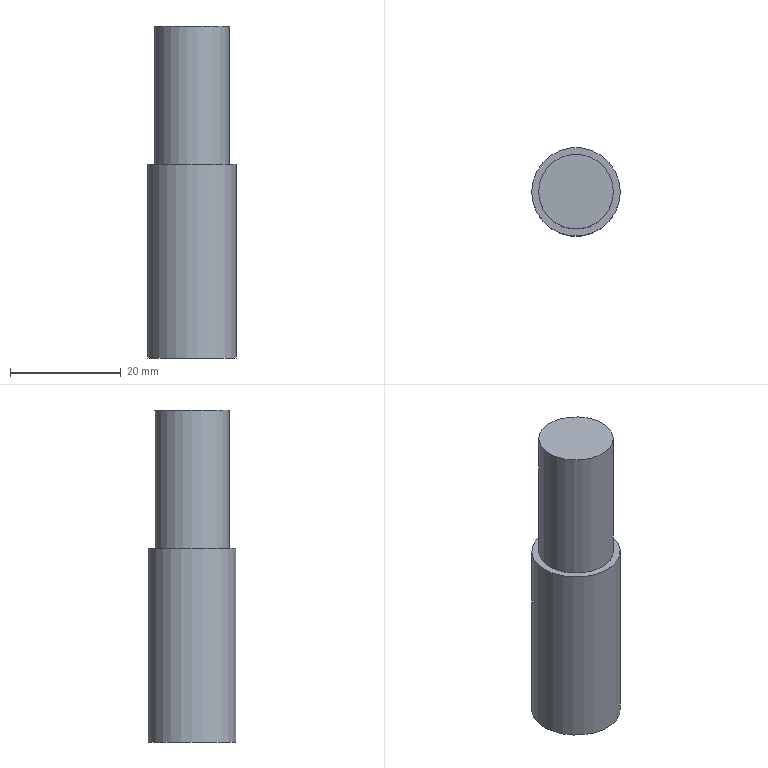Part | NX | features solid 2 | 1 solid | 9 faces | box 16 x 16 x 60 mm | volume 6437 mm3 | plane 5 | cylinder 4 | commonest cylinder face diameters 8 x1 10 x1 13.5 x1 16 x1
STEP:
#1=CARTESIAN_POINT('',(635.,-700.,-65.));
#2=VERTEX_POINT('',#1);
#3=CARTESIAN_POINT('',(630.,-700.,-65.));
#4=DIRECTION('',(0.,0.,1.));
#5=DIRECTION('',(1.,0.,0.));
#6=AXIS2_PLACEMENT_3D('',#3,#4,#5);
#7=CIRCLE('',#6,5.);
#8=EDGE_CURVE('',#2,#2,#7,.T.);
#9=ORIENTED_EDGE('',*,*,#8,.T.);
#10=EDGE_LOOP('',(#9));
#11=FACE_BOUND('',#10,.T.);
#12=CARTESIAN_POINT('',(635.,-700.,-115.));
#13=VERTEX_POINT('',#12);
#14=CARTESIAN_POINT('',(630.,-700.,-115.));
#15=DIRECTION('',(0.,0.,1.));
#16=DIRECTION('',(1.,0.,0.));
#17=AXIS2_PLACEMENT_3D('',#14,#15,#16);
#18=CIRCLE('',#17,5.);
#19=EDGE_CURVE('',#13,#13,#18,.T.);
#20=ORIENTED_EDGE('',*,*,#19,.F.);
#21=EDGE_LOOP('',(#20));
#22=FACE_BOUND('',#21,.T.);
#23=CARTESIAN_POINT('',(630.,-700.,-65.));
#24=DIRECTION('',(0.,0.,-1.));
#25=DIRECTION('',(1.,0.,0.));
#26=AXIS2_PLACEMENT_3D('',#23,#24,#25);
#27=CYLINDRICAL_SURFACE('',#26,5.);
#28=ADVANCED_FACE('',(#11,#22),#27,.F.);
#29=ORIENTED_EDGE('',*,*,#8,.F.);
#30=EDGE_LOOP('',(#29));
#31=FACE_BOUND('',#30,.T.);
#32=CARTESIAN_POINT('',(630.,-700.,-65.));
#33=DIRECTION('',(0.,0.,-1.));
#34=DIRECTION('',(1.,0.,0.));
#35=AXIS2_PLACEMENT_3D('',#32,#33,#34);
#36=PLANE('',#35);
#37=ADVANCED_FACE('',(#31),#36,.T.);
#38=CARTESIAN_POINT('',(634.,-700.,-115.));
#39=VERTEX_POINT('',#38);
#40=CARTESIAN_POINT('',(630.,-700.,-115.));
#41=DIRECTION('',(0.,0.,1.));
#42=DIRECTION('',(1.,0.,0.));
#43=AXIS2_PLACEMENT_3D('',#40,#41,#42);
#44=CIRCLE('',#43,4.);
#45=EDGE_CURVE('',#39,#39,#44,.T.);
#46=ORIENTED_EDGE('',*,*,#45,.F.);
#47=EDGE_LOOP('',(#46));
#48=FACE_BOUND('',#47,.T.);
#49=ORIENTED_EDGE('',*,*,#19,.T.);
#50=EDGE_LOOP('',(#49));
#51=FACE_BOUND('',#50,.T.);
#52=CARTESIAN_POINT('',(630.,-700.,-115.));
#53=DIRECTION('',(0.,0.,-1.));
#54=DIRECTION('',(1.,0.,0.));
#55=AXIS2_PLACEMENT_3D('',#52,#53,#54);
#56=PLANE('',#55);
#57=ADVANCED_FACE('',(#48,#51),#56,.F.);
#58=CARTESIAN_POINT('',(634.,-700.,-120.));
#59=VERTEX_POINT('',#58);
#60=CARTESIAN_POINT('',(630.,-700.,-120.));
#61=DIRECTION('',(0.,0.,1.));
#62=DIRECTION('',(1.,0.,0.));
#63=AXIS2_PLACEMENT_3D('',#60,#61,#62);
#64=CIRCLE('',#63,4.);
#65=EDGE_CURVE('',#59,#59,#64,.T.);
#66=ORIENTED_EDGE('',*,*,#65,.F.);
#67=EDGE_LOOP('',(#66));
#68=FACE_BOUND('',#67,.T.);
#69=ORIENTED_EDGE('',*,*,#45,.T.);
#70=EDGE_LOOP('',(#69));
#71=FACE_BOUND('',#70,.T.);
#72=CARTESIAN_POINT('',(630.,-700.,-110.));
#73=DIRECTION('',(0.,0.,-1.));
#74=DIRECTION('',(1.,0.,0.));
#75=AXIS2_PLACEMENT_3D('',#72,#73,#74);
#76=CYLINDRICAL_SURFACE('',#75,4.);
#77=ADVANCED_FACE('',(#68,#71),#76,.F.);
#78=CARTESIAN_POINT('',(623.25,-700.,-60.));
#79=VERTEX_POINT('',#78);
#80=CARTESIAN_POINT('',(630.,-700.,-60.));
#81=DIRECTION('',(0.,0.,-1.));
#82=DIRECTION('',(-1.,0.,0.));
#83=AXIS2_PLACEMENT_3D('',#80,#81,#82);
#84=CIRCLE('',#83,6.75);
#85=EDGE_CURVE('',#79,#79,#84,.F.);
#86=ORIENTED_EDGE('',*,*,#85,.F.);
#87=EDGE_LOOP('',(#86));
#88=FACE_BOUND('',#87,.T.);
#89=CARTESIAN_POINT('',(623.25,-700.,-85.));
#90=VERTEX_POINT('',#89);
#91=CARTESIAN_POINT('',(630.,-700.,-85.));
#92=DIRECTION('',(0.,0.,-1.));
#93=DIRECTION('',(-1.,0.,0.));
#94=AXIS2_PLACEMENT_3D('',#91,#92,#93);
#95=CIRCLE('',#94,6.75);
#96=EDGE_CURVE('',#90,#90,#95,.F.);
#97=ORIENTED_EDGE('',*,*,#96,.T.);
#98=EDGE_LOOP('',(#97));
#99=FACE_BOUND('',#98,.T.);
#100=CARTESIAN_POINT('',(630.,-700.,-60.));
#101=DIRECTION('',(0.,0.,-1.));
#102=DIRECTION('',(1.,0.,0.));
#103=AXIS2_PLACEMENT_3D('',#100,#101,#102);
#104=CYLINDRICAL_SURFACE('',#103,6.75);
#105=ADVANCED_FACE('',(#88,#99),#104,.T.);
#106=ORIENTED_EDGE('',*,*,#85,.T.);
#107=EDGE_LOOP('',(#106));
#108=FACE_BOUND('',#107,.T.);
#109=CARTESIAN_POINT('',(630.,-700.,-60.));
#110=DIRECTION('',(0.,0.,-1.));
#111=DIRECTION('',(1.,0.,0.));
#112=AXIS2_PLACEMENT_3D('',#109,#110,#111);
#113=PLANE('',#112);
#114=ADVANCED_FACE('',(#108),#113,.F.);
#115=CARTESIAN_POINT('',(638.,-700.,-85.));
#116=VERTEX_POINT('',#115);
#117=CARTESIAN_POINT('',(630.,-700.,-85.));
#118=DIRECTION('',(0.,0.,1.));
#119=DIRECTION('',(1.,0.,0.));
#120=AXIS2_PLACEMENT_3D('',#117,#118,#119);
#121=CIRCLE('',#120,8.);
#122=EDGE_CURVE('',#116,#116,#121,.T.);
#123=ORIENTED_EDGE('',*,*,#122,.F.);
#124=EDGE_LOOP('',(#123));
#125=FACE_BOUND('',#124,.T.);
#126=CARTESIAN_POINT('',(638.,-700.,-120.));
#127=VERTEX_POINT('',#126);
#128=CARTESIAN_POINT('',(630.,-700.,-120.));
#129=DIRECTION('',(0.,0.,1.));
#130=DIRECTION('',(1.,0.,0.));
#131=AXIS2_PLACEMENT_3D('',#128,#129,#130);
#132=CIRCLE('',#131,8.);
#133=EDGE_CURVE('',#127,#127,#132,.T.);
#134=ORIENTED_EDGE('',*,*,#133,.T.);
#135=EDGE_LOOP('',(#134));
#136=FACE_BOUND('',#135,.T.);
#137=CARTESIAN_POINT('',(630.,-700.,-85.));
#138=DIRECTION('',(0.,0.,-1.));
#139=DIRECTION('',(1.,0.,0.));
#140=AXIS2_PLACEMENT_3D('',#137,#138,#139);
#141=CYLINDRICAL_SURFACE('',#140,8.);
#142=ADVANCED_FACE('',(#125,#136),#141,.T.);
#143=ORIENTED_EDGE('',*,*,#96,.F.);
#144=EDGE_LOOP('',(#143));
#145=FACE_BOUND('',#144,.T.);
#146=ORIENTED_EDGE('',*,*,#122,.T.);
#147=EDGE_LOOP('',(#146));
#148=FACE_BOUND('',#147,.T.);
#149=CARTESIAN_POINT('',(630.,-700.,-85.));
#150=DIRECTION('',(0.,0.,-1.));
#151=DIRECTION('',(1.,0.,0.));
#152=AXIS2_PLACEMENT_3D('',#149,#150,#151);
#153=PLANE('',#152);
#154=ADVANCED_FACE('',(#145,#148),#153,.F.);
#155=ORIENTED_EDGE('',*,*,#65,.T.);
#156=EDGE_LOOP('',(#155));
#157=FACE_BOUND('',#156,.T.);
#158=ORIENTED_EDGE('',*,*,#133,.F.);
#159=EDGE_LOOP('',(#158));
#160=FACE_BOUND('',#159,.T.);
#161=CARTESIAN_POINT('',(630.,-700.,-120.));
#162=DIRECTION('',(0.,0.,-1.));
#163=DIRECTION('',(1.,0.,0.));
#164=AXIS2_PLACEMENT_3D('',#161,#162,#163);
#165=PLANE('',#164);
#166=ADVANCED_FACE('',(#157,#160),#165,.T.);
#167=CLOSED_SHELL('',(#28,#37,#57,#77,#105,#114,#142,#154,#166));
#168=MANIFOLD_SOLID_BREP('',#167);
#169=(LENGTH_UNIT()NAMED_UNIT(*)SI_UNIT(.MILLI.,.METRE.));
#170=UNCERTAINTY_MEASURE_WITH_UNIT(LENGTH_MEASURE(0.00001),#169,'','');
#171=(NAMED_UNIT(*)PLANE_ANGLE_UNIT()SI_UNIT($,.RADIAN.));
#172=(NAMED_UNIT(*)SI_UNIT($,.STERADIAN.)SOLID_ANGLE_UNIT());
#173=(GEOMETRIC_REPRESENTATION_CONTEXT(3)GLOBAL_UNCERTAINTY_ASSIGNED_CONTEXT((#170))GLOBAL_UNIT_ASSIGNED_CONTEXT((#169,#171,#172))REPRESENTATION_CONTEXT('',''));
#174=ADVANCED_BREP_SHAPE_REPRESENTATION('',(#168),#173);